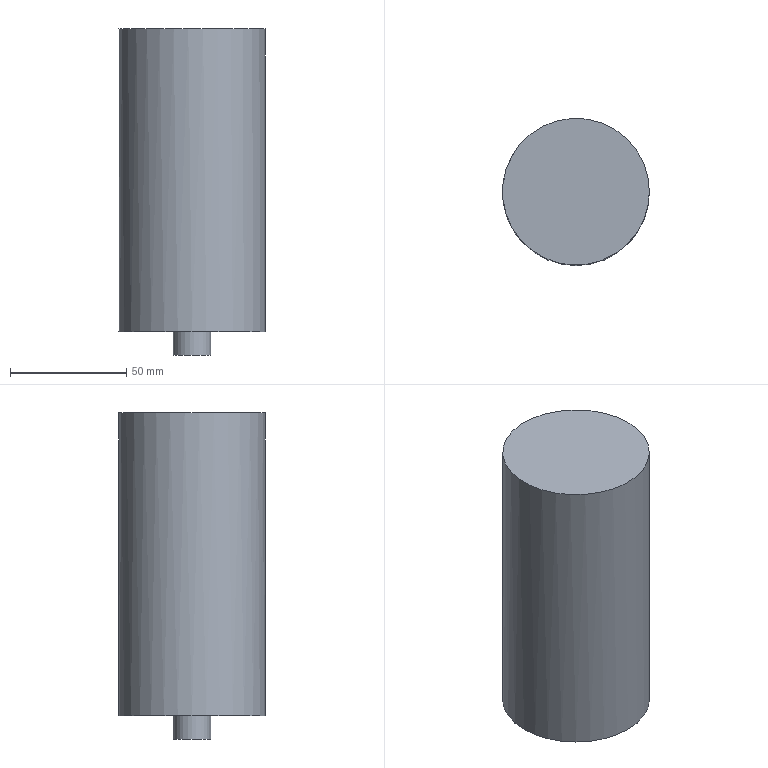Part | NX | features solid 2 | 1 solid | 5 faces | box 63 x 63 x 140 mm | volume 407253 mm3 | plane 3 | cylinder 2 | commonest cylinder face diameters 16 x1 63 x1
STEP:
#1=CARTESIAN_POINT('',(-693.5,193.5,250.));
#2=VERTEX_POINT('',#1);
#3=CARTESIAN_POINT('',(-725.,193.5,250.));
#4=DIRECTION('',(0.,0.,1.));
#5=DIRECTION('',(1.,0.,0.));
#6=AXIS2_PLACEMENT_3D('',#3,#4,#5);
#7=CIRCLE('',#6,31.5);
#8=EDGE_CURVE('',#2,#2,#7,.T.);
#9=ORIENTED_EDGE('',*,*,#8,.T.);
#10=EDGE_LOOP('',(#9));
#11=FACE_BOUND('',#10,.T.);
#12=CARTESIAN_POINT('',(-725.,193.5,250.));
#13=DIRECTION('',(0.,0.,1.));
#14=DIRECTION('',(1.,0.,0.));
#15=AXIS2_PLACEMENT_3D('',#12,#13,#14);
#16=PLANE('',#15);
#17=ADVANCED_FACE('',(#11),#16,.T.);
#18=CARTESIAN_POINT('',(-733.,193.5,120.));
#19=VERTEX_POINT('',#18);
#20=CARTESIAN_POINT('',(-725.,193.5,120.));
#21=DIRECTION('',(0.,0.,1.));
#22=DIRECTION('',(-1.,0.,0.));
#23=AXIS2_PLACEMENT_3D('',#20,#21,#22);
#24=CIRCLE('',#23,8.);
#25=EDGE_CURVE('',#19,#19,#24,.T.);
#26=ORIENTED_EDGE('',*,*,#25,.T.);
#27=EDGE_LOOP('',(#26));
#28=FACE_BOUND('',#27,.T.);
#29=CARTESIAN_POINT('',(-756.5,193.5,120.));
#30=VERTEX_POINT('',#29);
#31=CARTESIAN_POINT('',(-725.,193.5,120.));
#32=DIRECTION('',(0.,0.,1.));
#33=DIRECTION('',(-1.,0.,0.));
#34=AXIS2_PLACEMENT_3D('',#31,#32,#33);
#35=CIRCLE('',#34,31.5);
#36=EDGE_CURVE('',#30,#30,#35,.F.);
#37=ORIENTED_EDGE('',*,*,#36,.T.);
#38=EDGE_LOOP('',(#37));
#39=FACE_BOUND('',#38,.T.);
#40=CARTESIAN_POINT('',(-725.,193.5,120.));
#41=DIRECTION('',(0.,0.,-1.));
#42=DIRECTION('',(-1.,0.,0.));
#43=AXIS2_PLACEMENT_3D('',#40,#41,#42);
#44=PLANE('',#43);
#45=ADVANCED_FACE('',(#28,#39),#44,.T.);
#46=ORIENTED_EDGE('',*,*,#8,.F.);
#47=EDGE_LOOP('',(#46));
#48=FACE_BOUND('',#47,.T.);
#49=ORIENTED_EDGE('',*,*,#36,.F.);
#50=EDGE_LOOP('',(#49));
#51=FACE_BOUND('',#50,.T.);
#52=CARTESIAN_POINT('',(-725.,193.5,120.));
#53=DIRECTION('',(0.,0.,1.));
#54=DIRECTION('',(1.,0.,0.));
#55=AXIS2_PLACEMENT_3D('',#52,#53,#54);
#56=CYLINDRICAL_SURFACE('',#55,31.5);
#57=ADVANCED_FACE('',(#48,#51),#56,.T.);
#58=CARTESIAN_POINT('',(-717.,193.5,110.));
#59=VERTEX_POINT('',#58);
#60=CARTESIAN_POINT('',(-725.,193.5,110.));
#61=DIRECTION('',(0.,0.,-1.));
#62=DIRECTION('',(1.,0.,0.));
#63=AXIS2_PLACEMENT_3D('',#60,#61,#62);
#64=CIRCLE('',#63,8.);
#65=EDGE_CURVE('',#59,#59,#64,.T.);
#66=ORIENTED_EDGE('',*,*,#65,.T.);
#67=EDGE_LOOP('',(#66));
#68=FACE_BOUND('',#67,.T.);
#69=CARTESIAN_POINT('',(-725.,193.5,110.));
#70=DIRECTION('',(0.,0.,-1.));
#71=DIRECTION('',(-1.,0.,0.));
#72=AXIS2_PLACEMENT_3D('',#69,#70,#71);
#73=PLANE('',#72);
#74=ADVANCED_FACE('',(#68),#73,.T.);
#75=ORIENTED_EDGE('',*,*,#65,.F.);
#76=EDGE_LOOP('',(#75));
#77=FACE_BOUND('',#76,.T.);
#78=ORIENTED_EDGE('',*,*,#25,.F.);
#79=EDGE_LOOP('',(#78));
#80=FACE_BOUND('',#79,.T.);
#81=CARTESIAN_POINT('',(-725.,193.5,120.));
#82=DIRECTION('',(0.,0.,-1.));
#83=DIRECTION('',(-1.,0.,0.));
#84=AXIS2_PLACEMENT_3D('',#81,#82,#83);
#85=CYLINDRICAL_SURFACE('',#84,8.);
#86=ADVANCED_FACE('',(#77,#80),#85,.T.);
#87=CLOSED_SHELL('',(#17,#45,#57,#74,#86));
#88=MANIFOLD_SOLID_BREP('',#87);
#89=(LENGTH_UNIT()NAMED_UNIT(*)SI_UNIT(.MILLI.,.METRE.));
#90=UNCERTAINTY_MEASURE_WITH_UNIT(LENGTH_MEASURE(0.00001),#89,'','');
#91=(NAMED_UNIT(*)PLANE_ANGLE_UNIT()SI_UNIT($,.RADIAN.));
#92=(NAMED_UNIT(*)SI_UNIT($,.STERADIAN.)SOLID_ANGLE_UNIT());
#93=(GEOMETRIC_REPRESENTATION_CONTEXT(3)GLOBAL_UNCERTAINTY_ASSIGNED_CONTEXT((#90))GLOBAL_UNIT_ASSIGNED_CONTEXT((#89,#91,#92))REPRESENTATION_CONTEXT('',''));
#94=ADVANCED_BREP_SHAPE_REPRESENTATION('',(#88),#93);